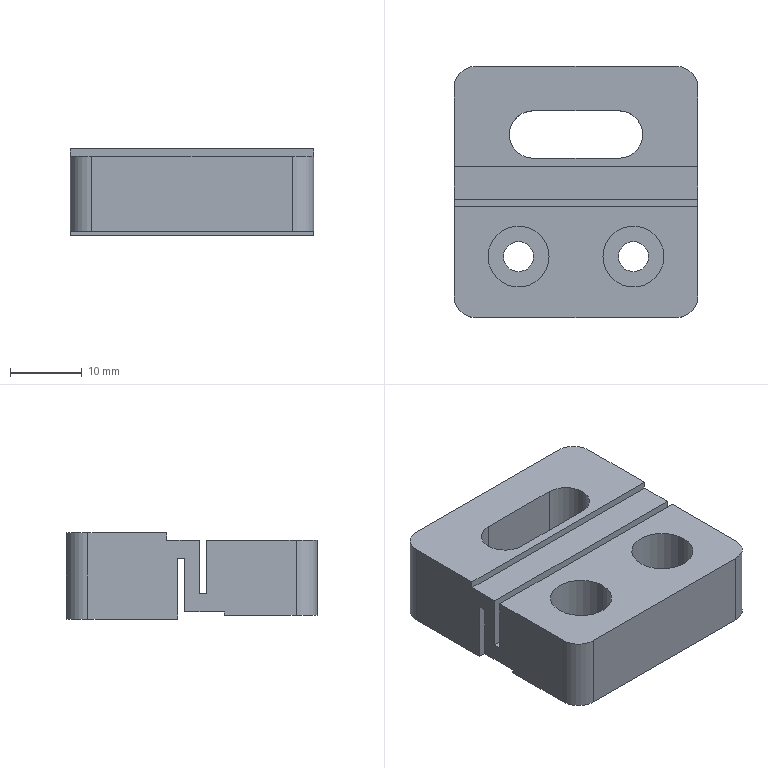Part | SolidWorks | features ICE 7, Extrusion 1, Fillet 1 | 1 solid | 37 faces | box 34 x 35 x 12 mm | volume 10318 mm3 | plane 22 | cylinder 15 | commonest cylinder face diameters 4.2 x4 6 x4 8.5 x4 6.6 x3
STEP:
#1=CARTESIAN_POINT('',(3.75,-9.,4.5));
#2=VERTEX_POINT('',#1);
#3=CARTESIAN_POINT('',(12.25,-9.,4.5));
#4=VERTEX_POINT('',#3);
#5=CARTESIAN_POINT('',(8.,-9.,4.5));
#6=DIRECTION('',(0.,0.,1.));
#7=DIRECTION('',(1.,0.,0.));
#8=AXIS2_PLACEMENT_3D('',#5,#6,#7);
#9=CIRCLE('',#8,4.25);
#10=EDGE_CURVE('',#2,#4,#9,.T.);
#11=ORIENTED_EDGE('',*,*,#10,.F.);
#12=CARTESIAN_POINT('',(3.75,-9.,11.));
#13=VERTEX_POINT('',#12);
#14=CARTESIAN_POINT('',(3.75,-9.,4.5));
#15=DIRECTION('',(0.,0.,1.));
#16=VECTOR('',#15,1000.);
#17=LINE('',#14,#16);
#18=EDGE_CURVE('',#2,#13,#17,.T.);
#19=ORIENTED_EDGE('',*,*,#18,.T.);
#20=CARTESIAN_POINT('',(12.25,-9.,11.));
#21=VERTEX_POINT('',#20);
#22=CARTESIAN_POINT('',(8.,-9.,11.));
#23=DIRECTION('',(0.,0.,1.));
#24=DIRECTION('',(1.,0.,0.));
#25=AXIS2_PLACEMENT_3D('',#22,#23,#24);
#26=CIRCLE('',#25,4.25);
#27=EDGE_CURVE('',#13,#21,#26,.T.);
#28=ORIENTED_EDGE('',*,*,#27,.T.);
#29=CARTESIAN_POINT('',(12.25,-9.,4.5));
#30=DIRECTION('',(0.,0.,1.));
#31=VECTOR('',#30,1000.);
#32=LINE('',#29,#31);
#33=EDGE_CURVE('',#4,#21,#32,.T.);
#34=ORIENTED_EDGE('',*,*,#33,.F.);
#35=EDGE_LOOP('',(#11,#19,#28,#34));
#36=FACE_OUTER_BOUND('',#35,.T.);
#37=CARTESIAN_POINT('',(8.,-9.,4.5));
#38=DIRECTION('',(0.,0.,1.));
#39=DIRECTION('',(1.,0.,0.));
#40=AXIS2_PLACEMENT_3D('',#37,#38,#39);
#41=CYLINDRICAL_SURFACE('',#40,4.25);
#42=ADVANCED_FACE('',(#36),#41,.F.);
#43=CARTESIAN_POINT('',(-12.25,-9.,4.5));
#44=VERTEX_POINT('',#43);
#45=CARTESIAN_POINT('',(-3.75,-9.,4.5));
#46=VERTEX_POINT('',#45);
#47=CARTESIAN_POINT('',(-8.,-9.,4.5));
#48=DIRECTION('',(0.,0.,1.));
#49=DIRECTION('',(1.,0.,0.));
#50=AXIS2_PLACEMENT_3D('',#47,#48,#49);
#51=CIRCLE('',#50,4.25);
#52=EDGE_CURVE('',#44,#46,#51,.T.);
#53=ORIENTED_EDGE('',*,*,#52,.F.);
#54=CARTESIAN_POINT('',(-12.25,-9.,11.));
#55=VERTEX_POINT('',#54);
#56=CARTESIAN_POINT('',(-12.25,-9.,4.5));
#57=DIRECTION('',(0.,0.,1.));
#58=VECTOR('',#57,1000.);
#59=LINE('',#56,#58);
#60=EDGE_CURVE('',#44,#55,#59,.T.);
#61=ORIENTED_EDGE('',*,*,#60,.T.);
#62=CARTESIAN_POINT('',(-3.75,-9.,11.));
#63=VERTEX_POINT('',#62);
#64=CARTESIAN_POINT('',(-8.,-9.,11.));
#65=DIRECTION('',(0.,0.,1.));
#66=DIRECTION('',(1.,0.,0.));
#67=AXIS2_PLACEMENT_3D('',#64,#65,#66);
#68=CIRCLE('',#67,4.25);
#69=EDGE_CURVE('',#55,#63,#68,.T.);
#70=ORIENTED_EDGE('',*,*,#69,.T.);
#71=CARTESIAN_POINT('',(-3.75,-9.,4.5));
#72=DIRECTION('',(0.,0.,1.));
#73=VECTOR('',#72,1000.);
#74=LINE('',#71,#73);
#75=EDGE_CURVE('',#46,#63,#74,.T.);
#76=ORIENTED_EDGE('',*,*,#75,.F.);
#77=EDGE_LOOP('',(#53,#61,#70,#76));
#78=FACE_OUTER_BOUND('',#77,.T.);
#79=CARTESIAN_POINT('',(-8.,-9.,4.5));
#80=DIRECTION('',(0.,0.,1.));
#81=DIRECTION('',(1.,0.,0.));
#82=AXIS2_PLACEMENT_3D('',#79,#80,#81);
#83=CYLINDRICAL_SURFACE('',#82,4.25);
#84=ADVANCED_FACE('',(#78),#83,.F.);
#85=CARTESIAN_POINT('',(9.3,8.,0.));
#86=VERTEX_POINT('',#85);
#87=CARTESIAN_POINT('',(6.,11.3,0.));
#88=VERTEX_POINT('',#87);
#89=CARTESIAN_POINT('',(6.,8.,0.));
#90=DIRECTION('',(0.,0.,1.));
#91=DIRECTION('',(1.,0.,0.));
#92=AXIS2_PLACEMENT_3D('',#89,#90,#91);
#93=CIRCLE('',#92,3.3);
#94=EDGE_CURVE('',#86,#88,#93,.T.);
#95=ORIENTED_EDGE('',*,*,#94,.F.);
#96=CARTESIAN_POINT('',(9.3,8.,12.));
#97=VERTEX_POINT('',#96);
#98=CARTESIAN_POINT('',(9.3,8.,0.));
#99=DIRECTION('',(0.,0.,1.));
#100=VECTOR('',#99,1000.);
#101=LINE('',#98,#100);
#102=EDGE_CURVE('',#86,#97,#101,.T.);
#103=ORIENTED_EDGE('',*,*,#102,.T.);
#104=CARTESIAN_POINT('',(6.,11.3,12.));
#105=VERTEX_POINT('',#104);
#106=CARTESIAN_POINT('',(6.,8.,12.));
#107=DIRECTION('',(0.,0.,1.));
#108=DIRECTION('',(1.,0.,0.));
#109=AXIS2_PLACEMENT_3D('',#106,#107,#108);
#110=CIRCLE('',#109,3.3);
#111=EDGE_CURVE('',#97,#105,#110,.T.);
#112=ORIENTED_EDGE('',*,*,#111,.T.);
#113=CARTESIAN_POINT('',(6.,11.3,0.));
#114=DIRECTION('',(0.,0.,1.));
#115=VECTOR('',#114,1000.);
#116=LINE('',#113,#115);
#117=EDGE_CURVE('',#88,#105,#116,.T.);
#118=ORIENTED_EDGE('',*,*,#117,.F.);
#119=EDGE_LOOP('',(#95,#103,#112,#118));
#120=FACE_OUTER_BOUND('',#119,.T.);
#121=CARTESIAN_POINT('',(6.,8.,0.));
#122=DIRECTION('',(0.,0.,1.));
#123=DIRECTION('',(1.,0.,0.));
#124=AXIS2_PLACEMENT_3D('',#121,#122,#123);
#125=CYLINDRICAL_SURFACE('',#124,3.3);
#126=ADVANCED_FACE('',(#120),#125,.F.);
#127=CARTESIAN_POINT('',(-5.9,-9.,0.5));
#128=VERTEX_POINT('',#127);
#129=CARTESIAN_POINT('',(-10.1,-9.,0.5));
#130=VERTEX_POINT('',#129);
#131=CARTESIAN_POINT('',(-8.,-9.,0.5));
#132=DIRECTION('',(0.,0.,-1.));
#133=DIRECTION('',(1.,0.,0.));
#134=AXIS2_PLACEMENT_3D('',#131,#132,#133);
#135=CIRCLE('',#134,2.1);
#136=EDGE_CURVE('',#128,#130,#135,.T.);
#137=ORIENTED_EDGE('',*,*,#136,.T.);
#138=CARTESIAN_POINT('',(-10.1,-9.,4.5));
#139=VERTEX_POINT('',#138);
#140=CARTESIAN_POINT('',(-10.1,-9.,0.));
#141=DIRECTION('',(0.,0.,1.));
#142=VECTOR('',#141,1000.);
#143=LINE('',#140,#142);
#144=EDGE_CURVE('',#130,#139,#143,.T.);
#145=ORIENTED_EDGE('',*,*,#144,.T.);
#146=CARTESIAN_POINT('',(-5.9,-9.,4.5));
#147=VERTEX_POINT('',#146);
#148=CARTESIAN_POINT('',(-8.,-9.,4.5));
#149=DIRECTION('',(0.,0.,-1.));
#150=DIRECTION('',(1.,0.,0.));
#151=AXIS2_PLACEMENT_3D('',#148,#149,#150);
#152=CIRCLE('',#151,2.1);
#153=EDGE_CURVE('',#147,#139,#152,.T.);
#154=ORIENTED_EDGE('',*,*,#153,.F.);
#155=CARTESIAN_POINT('',(-5.9,-9.,0.));
#156=DIRECTION('',(0.,0.,1.));
#157=VECTOR('',#156,1000.);
#158=LINE('',#155,#157);
#159=EDGE_CURVE('',#128,#147,#158,.T.);
#160=ORIENTED_EDGE('',*,*,#159,.F.);
#161=EDGE_LOOP('',(#137,#145,#154,#160));
#162=FACE_OUTER_BOUND('',#161,.T.);
#163=CARTESIAN_POINT('',(-8.,-9.,0.));
#164=DIRECTION('',(0.,0.,1.));
#165=DIRECTION('',(1.,0.,0.));
#166=AXIS2_PLACEMENT_3D('',#163,#164,#165);
#167=CYLINDRICAL_SURFACE('',#166,2.1);
#168=ADVANCED_FACE('',(#162),#167,.F.);
#169=CARTESIAN_POINT('',(10.1,-9.,0.5));
#170=VERTEX_POINT('',#169);
#171=CARTESIAN_POINT('',(5.9,-9.,0.5));
#172=VERTEX_POINT('',#171);
#173=CARTESIAN_POINT('',(8.,-9.,0.5));
#174=DIRECTION('',(0.,0.,-1.));
#175=DIRECTION('',(1.,0.,0.));
#176=AXIS2_PLACEMENT_3D('',#173,#174,#175);
#177=CIRCLE('',#176,2.1);
#178=EDGE_CURVE('',#170,#172,#177,.T.);
#179=ORIENTED_EDGE('',*,*,#178,.T.);
#180=CARTESIAN_POINT('',(5.9,-9.,4.5));
#181=VERTEX_POINT('',#180);
#182=CARTESIAN_POINT('',(5.9,-9.,0.));
#183=DIRECTION('',(0.,0.,1.));
#184=VECTOR('',#183,1000.);
#185=LINE('',#182,#184);
#186=EDGE_CURVE('',#172,#181,#185,.T.);
#187=ORIENTED_EDGE('',*,*,#186,.T.);
#188=CARTESIAN_POINT('',(10.1,-9.,4.5));
#189=VERTEX_POINT('',#188);
#190=CARTESIAN_POINT('',(8.,-9.,4.5));
#191=DIRECTION('',(0.,0.,-1.));
#192=DIRECTION('',(1.,0.,0.));
#193=AXIS2_PLACEMENT_3D('',#190,#191,#192);
#194=CIRCLE('',#193,2.1);
#195=EDGE_CURVE('',#189,#181,#194,.T.);
#196=ORIENTED_EDGE('',*,*,#195,.F.);
#197=CARTESIAN_POINT('',(10.1,-9.,0.));
#198=DIRECTION('',(0.,0.,1.));
#199=VECTOR('',#198,1000.);
#200=LINE('',#197,#199);
#201=EDGE_CURVE('',#170,#189,#200,.T.);
#202=ORIENTED_EDGE('',*,*,#201,.F.);
#203=EDGE_LOOP('',(#179,#187,#196,#202));
#204=FACE_OUTER_BOUND('',#203,.T.);
#205=CARTESIAN_POINT('',(8.,-9.,0.));
#206=DIRECTION('',(0.,0.,1.));
#207=DIRECTION('',(1.,0.,0.));
#208=AXIS2_PLACEMENT_3D('',#205,#206,#207);
#209=CYLINDRICAL_SURFACE('',#208,2.1);
#210=ADVANCED_FACE('',(#204),#209,.F.);
#211=CARTESIAN_POINT('',(-8.,-9.,11.));
#212=DIRECTION('',(0.,0.,1.));
#213=DIRECTION('',(1.,0.,0.));
#214=AXIS2_PLACEMENT_3D('',#211,#212,#213);
#215=CIRCLE('',#214,4.25);
#216=EDGE_CURVE('',#63,#55,#215,.T.);
#217=ORIENTED_EDGE('',*,*,#216,.F.);
#218=ORIENTED_EDGE('',*,*,#69,.F.);
#219=EDGE_LOOP('',(#217,#218));
#220=FACE_BOUND('',#219,.T.);
#221=CARTESIAN_POINT('',(8.,-9.,11.));
#222=DIRECTION('',(0.,0.,1.));
#223=DIRECTION('',(1.,0.,0.));
#224=AXIS2_PLACEMENT_3D('',#221,#222,#223);
#225=CIRCLE('',#224,4.25);
#226=EDGE_CURVE('',#21,#13,#225,.T.);
#227=ORIENTED_EDGE('',*,*,#226,.F.);
#228=ORIENTED_EDGE('',*,*,#27,.F.);
#229=EDGE_LOOP('',(#227,#228));
#230=FACE_BOUND('',#229,.T.);
#231=CARTESIAN_POINT('',(-17.,-14.5,11.));
#232=VERTEX_POINT('',#231);
#233=CARTESIAN_POINT('',(-17.,-2.,11.));
#234=VERTEX_POINT('',#233);
#235=CARTESIAN_POINT('',(-17.,-17.5,11.));
#236=DIRECTION('',(0.,1.,0.));
#237=VECTOR('',#236,1000.);
#238=LINE('',#235,#237);
#239=EDGE_CURVE('',#232,#234,#238,.T.);
#240=ORIENTED_EDGE('',*,*,#239,.F.);
#241=CARTESIAN_POINT('',(-14.,-17.5,11.));
#242=VERTEX_POINT('',#241);
#243=CARTESIAN_POINT('',(-14.,-14.5,11.));
#244=DIRECTION('',(0.,0.,1.));
#245=DIRECTION('',(-1.,0.,0.));
#246=AXIS2_PLACEMENT_3D('',#243,#244,#245);
#247=CIRCLE('',#246,3.);
#248=EDGE_CURVE('',#232,#242,#247,.T.);
#249=ORIENTED_EDGE('',*,*,#248,.T.);
#250=CARTESIAN_POINT('',(14.,-17.5,11.));
#251=VERTEX_POINT('',#250);
#252=CARTESIAN_POINT('',(17.,-17.5,11.));
#253=DIRECTION('',(-1.,0.,0.));
#254=VECTOR('',#253,1000.);
#255=LINE('',#252,#254);
#256=EDGE_CURVE('',#251,#242,#255,.T.);
#257=ORIENTED_EDGE('',*,*,#256,.F.);
#258=CARTESIAN_POINT('',(17.,-14.5,11.));
#259=VERTEX_POINT('',#258);
#260=CARTESIAN_POINT('',(14.,-14.5,11.));
#261=DIRECTION('',(0.,0.,1.));
#262=DIRECTION('',(-1.,0.,0.));
#263=AXIS2_PLACEMENT_3D('',#260,#261,#262);
#264=CIRCLE('',#263,3.);
#265=EDGE_CURVE('',#251,#259,#264,.T.);
#266=ORIENTED_EDGE('',*,*,#265,.T.);
#267=CARTESIAN_POINT('',(17.,-2.,11.));
#268=VERTEX_POINT('',#267);
#269=CARTESIAN_POINT('',(17.,-17.5,11.));
#270=DIRECTION('',(0.,-1.,0.));
#271=VECTOR('',#270,1000.);
#272=LINE('',#269,#271);
#273=EDGE_CURVE('',#268,#259,#272,.T.);
#274=ORIENTED_EDGE('',*,*,#273,.F.);
#275=CARTESIAN_POINT('',(17.,-2.,11.));
#276=DIRECTION('',(1.,0.,0.));
#277=VECTOR('',#276,1000.);
#278=LINE('',#275,#277);
#279=EDGE_CURVE('',#234,#268,#278,.T.);
#280=ORIENTED_EDGE('',*,*,#279,.F.);
#281=EDGE_LOOP('',(#240,#249,#257,#266,#274,#280));
#282=FACE_OUTER_BOUND('',#281,.T.);
#283=CARTESIAN_POINT('',(0.,0.,11.));
#284=DIRECTION('',(0.,0.,-1.));
#285=DIRECTION('',(-1.,0.,0.));
#286=AXIS2_PLACEMENT_3D('',#283,#284,#285);
#287=PLANE('',#286);
#288=ADVANCED_FACE('',(#220,#230,#282),#287,.F.);
#289=ORIENTED_EDGE('',*,*,#186,.F.);
#290=CARTESIAN_POINT('',(8.,-9.,0.5));
#291=DIRECTION('',(0.,0.,-1.));
#292=DIRECTION('',(1.,0.,0.));
#293=AXIS2_PLACEMENT_3D('',#290,#291,#292);
#294=CIRCLE('',#293,2.1);
#295=EDGE_CURVE('',#172,#170,#294,.T.);
#296=ORIENTED_EDGE('',*,*,#295,.T.);
#297=ORIENTED_EDGE('',*,*,#201,.T.);
#298=CARTESIAN_POINT('',(8.,-9.,4.5));
#299=DIRECTION('',(0.,0.,-1.));
#300=DIRECTION('',(1.,0.,0.));
#301=AXIS2_PLACEMENT_3D('',#298,#299,#300);
#302=CIRCLE('',#301,2.1);
#303=EDGE_CURVE('',#181,#189,#302,.T.);
#304=ORIENTED_EDGE('',*,*,#303,.F.);
#305=EDGE_LOOP('',(#289,#296,#297,#304));
#306=FACE_OUTER_BOUND('',#305,.T.);
#307=CARTESIAN_POINT('',(8.,-9.,0.));
#308=DIRECTION('',(0.,0.,1.));
#309=DIRECTION('',(1.,0.,0.));
#310=AXIS2_PLACEMENT_3D('',#307,#308,#309);
#311=CYLINDRICAL_SURFACE('',#310,2.1);
#312=ADVANCED_FACE('',(#306),#311,.F.);
#313=ORIENTED_EDGE('',*,*,#144,.F.);
#314=CARTESIAN_POINT('',(-8.,-9.,0.5));
#315=DIRECTION('',(0.,0.,-1.));
#316=DIRECTION('',(1.,0.,0.));
#317=AXIS2_PLACEMENT_3D('',#314,#315,#316);
#318=CIRCLE('',#317,2.1);
#319=EDGE_CURVE('',#130,#128,#318,.T.);
#320=ORIENTED_EDGE('',*,*,#319,.T.);
#321=ORIENTED_EDGE('',*,*,#159,.T.);
#322=CARTESIAN_POINT('',(-8.,-9.,4.5));
#323=DIRECTION('',(0.,0.,-1.));
#324=DIRECTION('',(1.,0.,0.));
#325=AXIS2_PLACEMENT_3D('',#322,#323,#324);
#326=CIRCLE('',#325,2.1);
#327=EDGE_CURVE('',#139,#147,#326,.T.);
#328=ORIENTED_EDGE('',*,*,#327,.F.);
#329=EDGE_LOOP('',(#313,#320,#321,#328));
#330=FACE_OUTER_BOUND('',#329,.T.);
#331=CARTESIAN_POINT('',(-8.,-9.,0.));
#332=DIRECTION('',(0.,0.,1.));
#333=DIRECTION('',(1.,0.,0.));
#334=AXIS2_PLACEMENT_3D('',#331,#332,#333);
#335=CYLINDRICAL_SURFACE('',#334,2.1);
#336=ADVANCED_FACE('',(#330),#335,.F.);
#337=CARTESIAN_POINT('',(-17.,-4.5,0.5));
#338=VERTEX_POINT('',#337);
#339=CARTESIAN_POINT('',(-17.,-14.5,0.5));
#340=VERTEX_POINT('',#339);
#341=CARTESIAN_POINT('',(-17.,-17.5,0.5));
#342=DIRECTION('',(0.,-1.,0.));
#343=VECTOR('',#342,1000.);
#344=LINE('',#341,#343);
#345=EDGE_CURVE('',#338,#340,#344,.T.);
#346=ORIENTED_EDGE('',*,*,#345,.T.);
#347=CARTESIAN_POINT('',(-17.,-14.5,12.));
#348=DIRECTION('',(0.,0.,1.));
#349=VECTOR('',#348,1000.);
#350=LINE('',#347,#349);
#351=EDGE_CURVE('',#340,#232,#350,.T.);
#352=ORIENTED_EDGE('',*,*,#351,.T.);
#353=ORIENTED_EDGE('',*,*,#239,.T.);
#354=CARTESIAN_POINT('',(-17.,-2.,3.5));
#355=VERTEX_POINT('',#354);
#356=CARTESIAN_POINT('',(-17.,-2.,-33.015));
#357=DIRECTION('',(0.,0.,1.));
#358=VECTOR('',#357,1000.);
#359=LINE('',#356,#358);
#360=EDGE_CURVE('',#355,#234,#359,.T.);
#361=ORIENTED_EDGE('',*,*,#360,.F.);
#362=CARTESIAN_POINT('',(-17.,-1.,3.5));
#363=VERTEX_POINT('',#362);
#364=CARTESIAN_POINT('',(-17.,-2.,3.5));
#365=DIRECTION('',(0.,1.,0.));
#366=VECTOR('',#365,1000.);
#367=LINE('',#364,#366);
#368=EDGE_CURVE('',#355,#363,#367,.T.);
#369=ORIENTED_EDGE('',*,*,#368,.T.);
#370=CARTESIAN_POINT('',(-17.,-1.,11.));
#371=VERTEX_POINT('',#370);
#372=CARTESIAN_POINT('',(-17.,-1.,-33.015));
#373=DIRECTION('',(0.,0.,1.));
#374=VECTOR('',#373,1000.);
#375=LINE('',#372,#374);
#376=EDGE_CURVE('',#363,#371,#375,.T.);
#377=ORIENTED_EDGE('',*,*,#376,.T.);
#378=CARTESIAN_POINT('',(-17.,3.5,11.));
#379=VERTEX_POINT('',#378);
#380=CARTESIAN_POINT('',(-17.,-17.5,11.));
#381=DIRECTION('',(0.,1.,0.));
#382=VECTOR('',#381,1000.);
#383=LINE('',#380,#382);
#384=EDGE_CURVE('',#371,#379,#383,.T.);
#385=ORIENTED_EDGE('',*,*,#384,.T.);
#386=CARTESIAN_POINT('',(-17.,3.5,12.));
#387=VERTEX_POINT('',#386);
#388=CARTESIAN_POINT('',(-17.,3.5,12.));
#389=DIRECTION('',(0.,0.,1.));
#390=VECTOR('',#389,1000.);
#391=LINE('',#388,#390);
#392=EDGE_CURVE('',#379,#387,#391,.T.);
#393=ORIENTED_EDGE('',*,*,#392,.T.);
#394=CARTESIAN_POINT('',(-17.,14.5,12.));
#395=VERTEX_POINT('',#394);
#396=CARTESIAN_POINT('',(-17.,-17.5,12.));
#397=DIRECTION('',(0.,-1.,0.));
#398=VECTOR('',#397,1000.);
#399=LINE('',#396,#398);
#400=EDGE_CURVE('',#395,#387,#399,.T.);
#401=ORIENTED_EDGE('',*,*,#400,.F.);
#402=CARTESIAN_POINT('',(-17.,14.5,0.));
#403=VERTEX_POINT('',#402);
#404=CARTESIAN_POINT('',(-17.,14.5,12.));
#405=DIRECTION('',(0.,0.,-1.));
#406=VECTOR('',#405,1000.);
#407=LINE('',#404,#406);
#408=EDGE_CURVE('',#395,#403,#407,.T.);
#409=ORIENTED_EDGE('',*,*,#408,.T.);
#410=CARTESIAN_POINT('',(-17.,2.,0.));
#411=VERTEX_POINT('',#410);
#412=CARTESIAN_POINT('',(-17.,-17.5,0.));
#413=DIRECTION('',(0.,-1.,0.));
#414=VECTOR('',#413,1000.);
#415=LINE('',#412,#414);
#416=EDGE_CURVE('',#403,#411,#415,.T.);
#417=ORIENTED_EDGE('',*,*,#416,.T.);
#418=CARTESIAN_POINT('',(-17.,2.,8.5));
#419=VERTEX_POINT('',#418);
#420=CARTESIAN_POINT('',(-17.,2.,12.));
#421=DIRECTION('',(0.,0.,1.));
#422=VECTOR('',#421,1000.);
#423=LINE('',#420,#422);
#424=EDGE_CURVE('',#411,#419,#423,.T.);
#425=ORIENTED_EDGE('',*,*,#424,.T.);
#426=CARTESIAN_POINT('',(-17.,1.,8.5));
#427=VERTEX_POINT('',#426);
#428=CARTESIAN_POINT('',(-17.,2.,8.5));
#429=DIRECTION('',(0.,-1.,0.));
#430=VECTOR('',#429,1000.);
#431=LINE('',#428,#430);
#432=EDGE_CURVE('',#419,#427,#431,.T.);
#433=ORIENTED_EDGE('',*,*,#432,.T.);
#434=CARTESIAN_POINT('',(-17.,1.,1.));
#435=VERTEX_POINT('',#434);
#436=CARTESIAN_POINT('',(-17.,1.,46.635));
#437=DIRECTION('',(0.,0.,-1.));
#438=VECTOR('',#437,1000.);
#439=LINE('',#436,#438);
#440=EDGE_CURVE('',#427,#435,#439,.T.);
#441=ORIENTED_EDGE('',*,*,#440,.T.);
#442=CARTESIAN_POINT('',(-17.,-4.5,1.));
#443=VERTEX_POINT('',#442);
#444=CARTESIAN_POINT('',(-17.,-17.5,1.));
#445=DIRECTION('',(0.,-1.,0.));
#446=VECTOR('',#445,1000.);
#447=LINE('',#444,#446);
#448=EDGE_CURVE('',#435,#443,#447,.T.);
#449=ORIENTED_EDGE('',*,*,#448,.T.);
#450=CARTESIAN_POINT('',(-17.,-4.5,1.));
#451=DIRECTION('',(0.,0.,-1.));
#452=VECTOR('',#451,1000.);
#453=LINE('',#450,#452);
#454=EDGE_CURVE('',#443,#338,#453,.T.);
#455=ORIENTED_EDGE('',*,*,#454,.T.);
#456=EDGE_LOOP('',(#346,#352,#353,#361,#369,#377,#385,#393,#401,#409,#417,#425,#433,#441,#449,#455));
#457=FACE_OUTER_BOUND('',#456,.T.);
#458=CARTESIAN_POINT('',(-17.,-17.5,12.));
#459=DIRECTION('',(1.,0.,0.));
#460=DIRECTION('',(0.,0.,-1.));
#461=AXIS2_PLACEMENT_3D('',#458,#459,#460);
#462=PLANE('',#461);
#463=ADVANCED_FACE('',(#457),#462,.F.);
#464=ORIENTED_EDGE('',*,*,#256,.T.);
#465=CARTESIAN_POINT('',(-14.,-17.5,0.5));
#466=VERTEX_POINT('',#465);
#467=CARTESIAN_POINT('',(-14.,-17.5,12.));
#468=DIRECTION('',(0.,0.,-1.));
#469=VECTOR('',#468,1000.);
#470=LINE('',#467,#469);
#471=EDGE_CURVE('',#242,#466,#470,.T.);
#472=ORIENTED_EDGE('',*,*,#471,.T.);
#473=CARTESIAN_POINT('',(14.,-17.5,0.5));
#474=VERTEX_POINT('',#473);
#475=CARTESIAN_POINT('',(17.,-17.5,0.5));
#476=DIRECTION('',(1.,0.,0.));
#477=VECTOR('',#476,1000.);
#478=LINE('',#475,#477);
#479=EDGE_CURVE('',#466,#474,#478,.T.);
#480=ORIENTED_EDGE('',*,*,#479,.T.);
#481=CARTESIAN_POINT('',(14.,-17.5,12.));
#482=DIRECTION('',(0.,0.,1.));
#483=VECTOR('',#482,1000.);
#484=LINE('',#481,#483);
#485=EDGE_CURVE('',#474,#251,#484,.T.);
#486=ORIENTED_EDGE('',*,*,#485,.T.);
#487=EDGE_LOOP('',(#464,#472,#480,#486));
#488=FACE_OUTER_BOUND('',#487,.T.);
#489=CARTESIAN_POINT('',(17.,-17.5,12.));
#490=DIRECTION('',(0.,1.,0.));
#491=DIRECTION('',(-1.,0.,0.));
#492=AXIS2_PLACEMENT_3D('',#489,#490,#491);
#493=PLANE('',#492);
#494=ADVANCED_FACE('',(#488),#493,.F.);
#495=ORIENTED_EDGE('',*,*,#273,.T.);
#496=CARTESIAN_POINT('',(17.,-14.5,0.5));
#497=VERTEX_POINT('',#496);
#498=CARTESIAN_POINT('',(17.,-14.5,12.));
#499=DIRECTION('',(0.,0.,-1.));
#500=VECTOR('',#499,1000.);
#501=LINE('',#498,#500);
#502=EDGE_CURVE('',#259,#497,#501,.T.);
#503=ORIENTED_EDGE('',*,*,#502,.T.);
#504=CARTESIAN_POINT('',(17.,-4.5,0.5));
#505=VERTEX_POINT('',#504);
#506=CARTESIAN_POINT('',(17.,-17.5,0.5));
#507=DIRECTION('',(0.,1.,0.));
#508=VECTOR('',#507,1000.);
#509=LINE('',#506,#508);
#510=EDGE_CURVE('',#497,#505,#509,.T.);
#511=ORIENTED_EDGE('',*,*,#510,.T.);
#512=CARTESIAN_POINT('',(17.,-4.5,1.));
#513=VERTEX_POINT('',#512);
#514=CARTESIAN_POINT('',(17.,-4.5,1.));
#515=DIRECTION('',(0.,0.,-1.));
#516=VECTOR('',#515,1000.);
#517=LINE('',#514,#516);
#518=EDGE_CURVE('',#513,#505,#517,.T.);
#519=ORIENTED_EDGE('',*,*,#518,.F.);
#520=CARTESIAN_POINT('',(17.,1.,1.));
#521=VERTEX_POINT('',#520);
#522=CARTESIAN_POINT('',(17.,-17.5,1.));
#523=DIRECTION('',(0.,1.,0.));
#524=VECTOR('',#523,1000.);
#525=LINE('',#522,#524);
#526=EDGE_CURVE('',#513,#521,#525,.T.);
#527=ORIENTED_EDGE('',*,*,#526,.T.);
#528=CARTESIAN_POINT('',(17.,1.,8.5));
#529=VERTEX_POINT('',#528);
#530=CARTESIAN_POINT('',(17.,1.,12.));
#531=DIRECTION('',(0.,0.,1.));
#532=VECTOR('',#531,1000.);
#533=LINE('',#530,#532);
#534=EDGE_CURVE('',#521,#529,#533,.T.);
#535=ORIENTED_EDGE('',*,*,#534,.T.);
#536=CARTESIAN_POINT('',(17.,2.,8.5));
#537=VERTEX_POINT('',#536);
#538=CARTESIAN_POINT('',(17.,-17.5,8.5));
#539=DIRECTION('',(0.,-1.,0.));
#540=VECTOR('',#539,1000.);
#541=LINE('',#538,#540);
#542=EDGE_CURVE('',#537,#529,#541,.T.);
#543=ORIENTED_EDGE('',*,*,#542,.F.);
#544=CARTESIAN_POINT('',(17.,2.,0.));
#545=VERTEX_POINT('',#544);
#546=CARTESIAN_POINT('',(17.,2.,12.));
#547=DIRECTION('',(0.,0.,-1.));
#548=VECTOR('',#547,1000.);
#549=LINE('',#546,#548);
#550=EDGE_CURVE('',#537,#545,#549,.T.);
#551=ORIENTED_EDGE('',*,*,#550,.T.);
#552=CARTESIAN_POINT('',(17.,14.5,0.));
#553=VERTEX_POINT('',#552);
#554=CARTESIAN_POINT('',(17.,-17.5,0.));
#555=DIRECTION('',(0.,1.,0.));
#556=VECTOR('',#555,1000.);
#557=LINE('',#554,#556);
#558=EDGE_CURVE('',#545,#553,#557,.T.);
#559=ORIENTED_EDGE('',*,*,#558,.T.);
#560=CARTESIAN_POINT('',(17.,14.5,12.));
#561=VERTEX_POINT('',#560);
#562=CARTESIAN_POINT('',(17.,14.5,12.));
#563=DIRECTION('',(0.,0.,1.));
#564=VECTOR('',#563,1000.);
#565=LINE('',#562,#564);
#566=EDGE_CURVE('',#553,#561,#565,.T.);
#567=ORIENTED_EDGE('',*,*,#566,.T.);
#568=CARTESIAN_POINT('',(17.,3.5,12.));
#569=VERTEX_POINT('',#568);
#570=CARTESIAN_POINT('',(17.,-17.5,12.));
#571=DIRECTION('',(0.,1.,0.));
#572=VECTOR('',#571,1000.);
#573=LINE('',#570,#572);
#574=EDGE_CURVE('',#569,#561,#573,.T.);
#575=ORIENTED_EDGE('',*,*,#574,.F.);
#576=CARTESIAN_POINT('',(17.,3.5,11.));
#577=VERTEX_POINT('',#576);
#578=CARTESIAN_POINT('',(17.,3.5,12.));
#579=DIRECTION('',(0.,0.,-1.));
#580=VECTOR('',#579,1000.);
#581=LINE('',#578,#580);
#582=EDGE_CURVE('',#569,#577,#581,.T.);
#583=ORIENTED_EDGE('',*,*,#582,.T.);
#584=CARTESIAN_POINT('',(17.,-1.,11.));
#585=VERTEX_POINT('',#584);
#586=CARTESIAN_POINT('',(17.,-17.5,11.));
#587=DIRECTION('',(0.,-1.,0.));
#588=VECTOR('',#587,1000.);
#589=LINE('',#586,#588);
#590=EDGE_CURVE('',#577,#585,#589,.T.);
#591=ORIENTED_EDGE('',*,*,#590,.T.);
#592=CARTESIAN_POINT('',(17.,-1.,3.5));
#593=VERTEX_POINT('',#592);
#594=CARTESIAN_POINT('',(17.,-1.,-33.015));
#595=DIRECTION('',(0.,0.,1.));
#596=VECTOR('',#595,1000.);
#597=LINE('',#594,#596);
#598=EDGE_CURVE('',#593,#585,#597,.T.);
#599=ORIENTED_EDGE('',*,*,#598,.F.);
#600=CARTESIAN_POINT('',(17.,-2.,3.5));
#601=VERTEX_POINT('',#600);
#602=CARTESIAN_POINT('',(17.,-1.,3.5));
#603=DIRECTION('',(0.,-1.,0.));
#604=VECTOR('',#603,1000.);
#605=LINE('',#602,#604);
#606=EDGE_CURVE('',#593,#601,#605,.T.);
#607=ORIENTED_EDGE('',*,*,#606,.T.);
#608=CARTESIAN_POINT('',(17.,-2.,-33.015));
#609=DIRECTION('',(0.,0.,1.));
#610=VECTOR('',#609,1000.);
#611=LINE('',#608,#610);
#612=EDGE_CURVE('',#601,#268,#611,.T.);
#613=ORIENTED_EDGE('',*,*,#612,.T.);
#614=EDGE_LOOP('',(#495,#503,#511,#519,#527,#535,#543,#551,#559,#567,#575,#583,#591,#599,#607,#613));
#615=FACE_OUTER_BOUND('',#614,.T.);
#616=CARTESIAN_POINT('',(17.,-17.5,12.));
#617=DIRECTION('',(-1.,0.,0.));
#618=DIRECTION('',(0.,0.,1.));
#619=AXIS2_PLACEMENT_3D('',#616,#617,#618);
#620=PLANE('',#619);
#621=ADVANCED_FACE('',(#615),#620,.F.);
#622=CARTESIAN_POINT('',(14.,17.5,12.));
#623=VERTEX_POINT('',#622);
#624=CARTESIAN_POINT('',(-14.,17.5,12.));
#625=VERTEX_POINT('',#624);
#626=CARTESIAN_POINT('',(17.,17.5,12.));
#627=DIRECTION('',(-1.,0.,0.));
#628=VECTOR('',#627,1000.);
#629=LINE('',#626,#628);
#630=EDGE_CURVE('',#623,#625,#629,.T.);
#631=ORIENTED_EDGE('',*,*,#630,.F.);
#632=CARTESIAN_POINT('',(14.,17.5,0.));
#633=VERTEX_POINT('',#632);
#634=CARTESIAN_POINT('',(14.,17.5,12.));
#635=DIRECTION('',(0.,0.,-1.));
#636=VECTOR('',#635,1000.);
#637=LINE('',#634,#636);
#638=EDGE_CURVE('',#623,#633,#637,.T.);
#639=ORIENTED_EDGE('',*,*,#638,.T.);
#640=CARTESIAN_POINT('',(-14.,17.5,0.));
#641=VERTEX_POINT('',#640);
#642=CARTESIAN_POINT('',(17.,17.5,0.));
#643=DIRECTION('',(-1.,0.,0.));
#644=VECTOR('',#643,1000.);
#645=LINE('',#642,#644);
#646=EDGE_CURVE('',#633,#641,#645,.T.);
#647=ORIENTED_EDGE('',*,*,#646,.T.);
#648=CARTESIAN_POINT('',(-14.,17.5,12.));
#649=DIRECTION('',(0.,0.,1.));
#650=VECTOR('',#649,1000.);
#651=LINE('',#648,#650);
#652=EDGE_CURVE('',#641,#625,#651,.T.);
#653=ORIENTED_EDGE('',*,*,#652,.T.);
#654=EDGE_LOOP('',(#631,#639,#647,#653));
#655=FACE_OUTER_BOUND('',#654,.T.);
#656=CARTESIAN_POINT('',(17.,17.5,12.));
#657=DIRECTION('',(0.,-1.,0.));
#658=DIRECTION('',(0.,0.,-1.));
#659=AXIS2_PLACEMENT_3D('',#656,#657,#658);
#660=PLANE('',#659);
#661=ADVANCED_FACE('',(#655),#660,.F.);
#662=ORIENTED_EDGE('',*,*,#574,.T.);
#663=CARTESIAN_POINT('',(14.,14.5,12.));
#664=DIRECTION('',(0.,0.,1.));
#665=DIRECTION('',(1.,0.,0.));
#666=AXIS2_PLACEMENT_3D('',#663,#664,#665);
#667=CIRCLE('',#666,3.);
#668=EDGE_CURVE('',#561,#623,#667,.T.);
#669=ORIENTED_EDGE('',*,*,#668,.T.);
#670=ORIENTED_EDGE('',*,*,#630,.T.);
#671=CARTESIAN_POINT('',(-14.,14.5,12.));
#672=DIRECTION('',(0.,0.,1.));
#673=DIRECTION('',(1.,0.,0.));
#674=AXIS2_PLACEMENT_3D('',#671,#672,#673);
#675=CIRCLE('',#674,3.);
#676=EDGE_CURVE('',#625,#395,#675,.T.);
#677=ORIENTED_EDGE('',*,*,#676,.T.);
#678=ORIENTED_EDGE('',*,*,#400,.T.);
#679=CARTESIAN_POINT('',(-20.364,3.5,12.));
#680=DIRECTION('',(-1.,0.,0.));
#681=VECTOR('',#680,1000.);
#682=LINE('',#679,#681);
#683=EDGE_CURVE('',#569,#387,#682,.T.);
#684=ORIENTED_EDGE('',*,*,#683,.F.);
#685=EDGE_LOOP('',(#662,#669,#670,#677,#678,#684));
#686=FACE_OUTER_BOUND('',#685,.T.);
#687=CARTESIAN_POINT('',(-6.,11.3,12.));
#688=VERTEX_POINT('',#687);
#689=CARTESIAN_POINT('',(-6.,4.7,12.));
#690=VERTEX_POINT('',#689);
#691=CARTESIAN_POINT('',(-6.,8.,12.));
#692=DIRECTION('',(0.,0.,1.));
#693=DIRECTION('',(1.,0.,0.));
#694=AXIS2_PLACEMENT_3D('',#691,#692,#693);
#695=CIRCLE('',#694,3.3);
#696=EDGE_CURVE('',#688,#690,#695,.T.);
#697=ORIENTED_EDGE('',*,*,#696,.F.);
#698=CARTESIAN_POINT('',(-6.,11.3,12.));
#699=DIRECTION('',(-1.,0.,0.));
#700=VECTOR('',#699,1000.);
#701=LINE('',#698,#700);
#702=EDGE_CURVE('',#105,#688,#701,.T.);
#703=ORIENTED_EDGE('',*,*,#702,.F.);
#704=ORIENTED_EDGE('',*,*,#111,.F.);
#705=CARTESIAN_POINT('',(6.,4.7,12.));
#706=VERTEX_POINT('',#705);
#707=CARTESIAN_POINT('',(6.,8.,12.));
#708=DIRECTION('',(0.,0.,1.));
#709=DIRECTION('',(1.,0.,0.));
#710=AXIS2_PLACEMENT_3D('',#707,#708,#709);
#711=CIRCLE('',#710,3.3);
#712=EDGE_CURVE('',#706,#97,#711,.T.);
#713=ORIENTED_EDGE('',*,*,#712,.F.);
#714=CARTESIAN_POINT('',(-6.,4.7,12.));
#715=DIRECTION('',(1.,0.,0.));
#716=VECTOR('',#715,1000.);
#717=LINE('',#714,#716);
#718=EDGE_CURVE('',#690,#706,#717,.T.);
#719=ORIENTED_EDGE('',*,*,#718,.F.);
#720=EDGE_LOOP('',(#697,#703,#704,#713,#719));
#721=FACE_BOUND('',#720,.T.);
#722=CARTESIAN_POINT('',(0.,0.,12.));
#723=DIRECTION('',(0.,0.,1.));
#724=DIRECTION('',(1.,0.,0.));
#725=AXIS2_PLACEMENT_3D('',#722,#723,#724);
#726=PLANE('',#725);
#727=ADVANCED_FACE('',(#686,#721),#726,.T.);
#728=CARTESIAN_POINT('',(-6.,11.3,0.));
#729=VERTEX_POINT('',#728);
#730=CARTESIAN_POINT('',(-6.,11.3,0.));
#731=DIRECTION('',(-1.,0.,0.));
#732=VECTOR('',#731,1000.);
#733=LINE('',#730,#732);
#734=EDGE_CURVE('',#88,#729,#733,.T.);
#735=ORIENTED_EDGE('',*,*,#734,.T.);
#736=CARTESIAN_POINT('',(-6.,4.7,0.));
#737=VERTEX_POINT('',#736);
#738=CARTESIAN_POINT('',(-6.,8.,0.));
#739=DIRECTION('',(0.,0.,1.));
#740=DIRECTION('',(1.,0.,0.));
#741=AXIS2_PLACEMENT_3D('',#738,#739,#740);
#742=CIRCLE('',#741,3.3);
#743=EDGE_CURVE('',#729,#737,#742,.T.);
#744=ORIENTED_EDGE('',*,*,#743,.T.);
#745=CARTESIAN_POINT('',(6.,4.7,0.));
#746=VERTEX_POINT('',#745);
#747=CARTESIAN_POINT('',(-6.,4.7,0.));
#748=DIRECTION('',(1.,0.,0.));
#749=VECTOR('',#748,1000.);
#750=LINE('',#747,#749);
#751=EDGE_CURVE('',#737,#746,#750,.T.);
#752=ORIENTED_EDGE('',*,*,#751,.T.);
#753=CARTESIAN_POINT('',(6.,8.,0.));
#754=DIRECTION('',(0.,0.,1.));
#755=DIRECTION('',(1.,0.,0.));
#756=AXIS2_PLACEMENT_3D('',#753,#754,#755);
#757=CIRCLE('',#756,3.3);
#758=EDGE_CURVE('',#746,#86,#757,.T.);
#759=ORIENTED_EDGE('',*,*,#758,.T.);
#760=ORIENTED_EDGE('',*,*,#94,.T.);
#761=EDGE_LOOP('',(#735,#744,#752,#759,#760));
#762=FACE_BOUND('',#761,.T.);
#763=ORIENTED_EDGE('',*,*,#646,.F.);
#764=CARTESIAN_POINT('',(14.,14.5,0.));
#765=DIRECTION('',(0.,0.,-1.));
#766=DIRECTION('',(1.,0.,0.));
#767=AXIS2_PLACEMENT_3D('',#764,#765,#766);
#768=CIRCLE('',#767,3.);
#769=EDGE_CURVE('',#633,#553,#768,.T.);
#770=ORIENTED_EDGE('',*,*,#769,.T.);
#771=ORIENTED_EDGE('',*,*,#558,.F.);
#772=CARTESIAN_POINT('',(23.913,2.,0.));
#773=DIRECTION('',(1.,0.,0.));
#774=VECTOR('',#773,1000.);
#775=LINE('',#772,#774);
#776=EDGE_CURVE('',#411,#545,#775,.T.);
#777=ORIENTED_EDGE('',*,*,#776,.F.);
#778=ORIENTED_EDGE('',*,*,#416,.F.);
#779=CARTESIAN_POINT('',(-14.,14.5,0.));
#780=DIRECTION('',(0.,0.,-1.));
#781=DIRECTION('',(1.,0.,0.));
#782=AXIS2_PLACEMENT_3D('',#779,#780,#781);
#783=CIRCLE('',#782,3.);
#784=EDGE_CURVE('',#403,#641,#783,.T.);
#785=ORIENTED_EDGE('',*,*,#784,.T.);
#786=EDGE_LOOP('',(#763,#770,#771,#777,#778,#785));
#787=FACE_OUTER_BOUND('',#786,.T.);
#788=CARTESIAN_POINT('',(0.,0.,0.));
#789=DIRECTION('',(0.,0.,1.));
#790=DIRECTION('',(1.,0.,0.));
#791=AXIS2_PLACEMENT_3D('',#788,#789,#790);
#792=PLANE('',#791);
#793=ADVANCED_FACE('',(#762,#787),#792,.F.);
#794=ORIENTED_EDGE('',*,*,#696,.T.);
#795=CARTESIAN_POINT('',(-6.,4.7,0.));
#796=DIRECTION('',(0.,0.,1.));
#797=VECTOR('',#796,1000.);
#798=LINE('',#795,#797);
#799=EDGE_CURVE('',#737,#690,#798,.T.);
#800=ORIENTED_EDGE('',*,*,#799,.F.);
#801=ORIENTED_EDGE('',*,*,#743,.F.);
#802=CARTESIAN_POINT('',(-6.,11.3,0.));
#803=DIRECTION('',(0.,0.,1.));
#804=VECTOR('',#803,1000.);
#805=LINE('',#802,#804);
#806=EDGE_CURVE('',#729,#688,#805,.T.);
#807=ORIENTED_EDGE('',*,*,#806,.T.);
#808=EDGE_LOOP('',(#794,#800,#801,#807));
#809=FACE_OUTER_BOUND('',#808,.T.);
#810=CARTESIAN_POINT('',(-6.,8.,0.));
#811=DIRECTION('',(0.,0.,1.));
#812=DIRECTION('',(1.,0.,0.));
#813=AXIS2_PLACEMENT_3D('',#810,#811,#812);
#814=CYLINDRICAL_SURFACE('',#813,3.3);
#815=ADVANCED_FACE('',(#809),#814,.F.);
#816=ORIENTED_EDGE('',*,*,#702,.T.);
#817=ORIENTED_EDGE('',*,*,#806,.F.);
#818=ORIENTED_EDGE('',*,*,#734,.F.);
#819=ORIENTED_EDGE('',*,*,#117,.T.);
#820=EDGE_LOOP('',(#816,#817,#818,#819));
#821=FACE_OUTER_BOUND('',#820,.T.);
#822=CARTESIAN_POINT('',(-6.,11.3,0.));
#823=DIRECTION('',(0.,1.,0.));
#824=DIRECTION('',(0.,0.,1.));
#825=AXIS2_PLACEMENT_3D('',#822,#823,#824);
#826=PLANE('',#825);
#827=ADVANCED_FACE('',(#821),#826,.F.);
#828=ORIENTED_EDGE('',*,*,#102,.F.);
#829=ORIENTED_EDGE('',*,*,#758,.F.);
#830=CARTESIAN_POINT('',(6.,4.7,0.));
#831=DIRECTION('',(0.,0.,1.));
#832=VECTOR('',#831,1000.);
#833=LINE('',#830,#832);
#834=EDGE_CURVE('',#746,#706,#833,.T.);
#835=ORIENTED_EDGE('',*,*,#834,.T.);
#836=ORIENTED_EDGE('',*,*,#712,.T.);
#837=EDGE_LOOP('',(#828,#829,#835,#836));
#838=FACE_OUTER_BOUND('',#837,.T.);
#839=CARTESIAN_POINT('',(6.,8.,0.));
#840=DIRECTION('',(0.,0.,1.));
#841=DIRECTION('',(1.,0.,0.));
#842=AXIS2_PLACEMENT_3D('',#839,#840,#841);
#843=CYLINDRICAL_SURFACE('',#842,3.3);
#844=ADVANCED_FACE('',(#838),#843,.F.);
#845=ORIENTED_EDGE('',*,*,#718,.T.);
#846=ORIENTED_EDGE('',*,*,#834,.F.);
#847=ORIENTED_EDGE('',*,*,#751,.F.);
#848=ORIENTED_EDGE('',*,*,#799,.T.);
#849=EDGE_LOOP('',(#845,#846,#847,#848));
#850=FACE_OUTER_BOUND('',#849,.T.);
#851=CARTESIAN_POINT('',(-6.,4.7,0.));
#852=DIRECTION('',(0.,-1.,0.));
#853=DIRECTION('',(0.,0.,-1.));
#854=AXIS2_PLACEMENT_3D('',#851,#852,#853);
#855=PLANE('',#854);
#856=ADVANCED_FACE('',(#850),#855,.F.);
#857=CARTESIAN_POINT('',(-20.364,3.5,11.));
#858=DIRECTION('',(-1.,0.,0.));
#859=VECTOR('',#858,1000.);
#860=LINE('',#857,#859);
#861=EDGE_CURVE('',#577,#379,#860,.T.);
#862=ORIENTED_EDGE('',*,*,#861,.F.);
#863=ORIENTED_EDGE('',*,*,#582,.F.);
#864=ORIENTED_EDGE('',*,*,#683,.T.);
#865=ORIENTED_EDGE('',*,*,#392,.F.);
#866=EDGE_LOOP('',(#862,#863,#864,#865));
#867=FACE_OUTER_BOUND('',#866,.T.);
#868=CARTESIAN_POINT('',(-20.364,3.5,11.));
#869=DIRECTION('',(0.,1.,0.));
#870=DIRECTION('',(0.,0.,1.));
#871=AXIS2_PLACEMENT_3D('',#868,#869,#870);
#872=PLANE('',#871);
#873=ADVANCED_FACE('',(#867),#872,.F.);
#874=ORIENTED_EDGE('',*,*,#384,.F.);
#875=CARTESIAN_POINT('',(-17.,-1.,11.));
#876=DIRECTION('',(-1.,0.,0.));
#877=VECTOR('',#876,1000.);
#878=LINE('',#875,#877);
#879=EDGE_CURVE('',#585,#371,#878,.T.);
#880=ORIENTED_EDGE('',*,*,#879,.F.);
#881=ORIENTED_EDGE('',*,*,#590,.F.);
#882=ORIENTED_EDGE('',*,*,#861,.T.);
#883=EDGE_LOOP('',(#874,#880,#881,#882));
#884=FACE_OUTER_BOUND('',#883,.T.);
#885=CARTESIAN_POINT('',(0.,0.,11.));
#886=DIRECTION('',(0.,0.,-1.));
#887=DIRECTION('',(-1.,0.,0.));
#888=AXIS2_PLACEMENT_3D('',#885,#886,#887);
#889=PLANE('',#888);
#890=ADVANCED_FACE('',(#884),#889,.F.);
#891=ORIENTED_EDGE('',*,*,#136,.F.);
#892=ORIENTED_EDGE('',*,*,#319,.F.);
#893=EDGE_LOOP('',(#891,#892));
#894=FACE_BOUND('',#893,.T.);
#895=ORIENTED_EDGE('',*,*,#178,.F.);
#896=ORIENTED_EDGE('',*,*,#295,.F.);
#897=EDGE_LOOP('',(#895,#896));
#898=FACE_BOUND('',#897,.T.);
#899=ORIENTED_EDGE('',*,*,#479,.F.);
#900=CARTESIAN_POINT('',(-14.,-14.5,0.5));
#901=DIRECTION('',(0.,0.,-1.));
#902=DIRECTION('',(1.,0.,0.));
#903=AXIS2_PLACEMENT_3D('',#900,#901,#902);
#904=CIRCLE('',#903,3.);
#905=EDGE_CURVE('',#466,#340,#904,.T.);
#906=ORIENTED_EDGE('',*,*,#905,.T.);
#907=ORIENTED_EDGE('',*,*,#345,.F.);
#908=CARTESIAN_POINT('',(24.763,-4.5,0.5));
#909=DIRECTION('',(1.,0.,0.));
#910=VECTOR('',#909,1000.);
#911=LINE('',#908,#910);
#912=EDGE_CURVE('',#338,#505,#911,.T.);
#913=ORIENTED_EDGE('',*,*,#912,.T.);
#914=ORIENTED_EDGE('',*,*,#510,.F.);
#915=CARTESIAN_POINT('',(14.,-14.5,0.5));
#916=DIRECTION('',(0.,0.,-1.));
#917=DIRECTION('',(1.,0.,0.));
#918=AXIS2_PLACEMENT_3D('',#915,#916,#917);
#919=CIRCLE('',#918,3.);
#920=EDGE_CURVE('',#497,#474,#919,.T.);
#921=ORIENTED_EDGE('',*,*,#920,.T.);
#922=EDGE_LOOP('',(#899,#906,#907,#913,#914,#921));
#923=FACE_OUTER_BOUND('',#922,.T.);
#924=CARTESIAN_POINT('',(0.,0.,0.5));
#925=DIRECTION('',(0.,0.,1.));
#926=DIRECTION('',(1.,0.,0.));
#927=AXIS2_PLACEMENT_3D('',#924,#925,#926);
#928=PLANE('',#927);
#929=ADVANCED_FACE('',(#894,#898,#923),#928,.F.);
#930=ORIENTED_EDGE('',*,*,#448,.F.);
#931=CARTESIAN_POINT('',(-17.,1.,1.));
#932=DIRECTION('',(-1.,0.,0.));
#933=VECTOR('',#932,1000.);
#934=LINE('',#931,#933);
#935=EDGE_CURVE('',#521,#435,#934,.T.);
#936=ORIENTED_EDGE('',*,*,#935,.F.);
#937=ORIENTED_EDGE('',*,*,#526,.F.);
#938=CARTESIAN_POINT('',(-17.,-4.5,1.));
#939=DIRECTION('',(-1.,0.,0.));
#940=VECTOR('',#939,1000.);
#941=LINE('',#938,#940);
#942=EDGE_CURVE('',#513,#443,#941,.T.);
#943=ORIENTED_EDGE('',*,*,#942,.T.);
#944=EDGE_LOOP('',(#930,#936,#937,#943));
#945=FACE_OUTER_BOUND('',#944,.T.);
#946=CARTESIAN_POINT('',(0.,0.,1.));
#947=DIRECTION('',(0.,0.,1.));
#948=DIRECTION('',(1.,0.,0.));
#949=AXIS2_PLACEMENT_3D('',#946,#947,#948);
#950=PLANE('',#949);
#951=ADVANCED_FACE('',(#945),#950,.F.);
#952=ORIENTED_EDGE('',*,*,#776,.T.);
#953=ORIENTED_EDGE('',*,*,#550,.F.);
#954=CARTESIAN_POINT('',(18.621,2.,8.5));
#955=DIRECTION('',(-1.,0.,0.));
#956=VECTOR('',#955,1000.);
#957=LINE('',#954,#956);
#958=EDGE_CURVE('',#537,#419,#957,.T.);
#959=ORIENTED_EDGE('',*,*,#958,.T.);
#960=ORIENTED_EDGE('',*,*,#424,.F.);
#961=EDGE_LOOP('',(#952,#953,#959,#960));
#962=FACE_OUTER_BOUND('',#961,.T.);
#963=CARTESIAN_POINT('',(23.913,2.,1.));
#964=DIRECTION('',(0.,1.,0.));
#965=DIRECTION('',(0.,0.,1.));
#966=AXIS2_PLACEMENT_3D('',#963,#964,#965);
#967=PLANE('',#966);
#968=ADVANCED_FACE('',(#962),#967,.F.);
#969=ORIENTED_EDGE('',*,*,#454,.F.);
#970=ORIENTED_EDGE('',*,*,#942,.F.);
#971=ORIENTED_EDGE('',*,*,#518,.T.);
#972=ORIENTED_EDGE('',*,*,#912,.F.);
#973=EDGE_LOOP('',(#969,#970,#971,#972));
#974=FACE_OUTER_BOUND('',#973,.T.);
#975=CARTESIAN_POINT('',(-17.,-4.5,1.));
#976=DIRECTION('',(0.,-1.,0.));
#977=DIRECTION('',(0.,0.,-1.));
#978=AXIS2_PLACEMENT_3D('',#975,#976,#977);
#979=PLANE('',#978);
#980=ADVANCED_FACE('',(#974),#979,.F.);
#981=CARTESIAN_POINT('',(-8.,-9.,4.5));
#982=DIRECTION('',(0.,0.,1.));
#983=DIRECTION('',(1.,0.,0.));
#984=AXIS2_PLACEMENT_3D('',#981,#982,#983);
#985=CIRCLE('',#984,4.25);
#986=EDGE_CURVE('',#46,#44,#985,.T.);
#987=ORIENTED_EDGE('',*,*,#986,.T.);
#988=ORIENTED_EDGE('',*,*,#52,.T.);
#989=EDGE_LOOP('',(#987,#988));
#990=FACE_OUTER_BOUND('',#989,.T.);
#991=ORIENTED_EDGE('',*,*,#153,.T.);
#992=ORIENTED_EDGE('',*,*,#327,.T.);
#993=EDGE_LOOP('',(#991,#992));
#994=FACE_BOUND('',#993,.T.);
#995=CARTESIAN_POINT('',(-8.,-9.,4.5));
#996=DIRECTION('',(0.,0.,1.));
#997=DIRECTION('',(1.,0.,0.));
#998=AXIS2_PLACEMENT_3D('',#995,#996,#997);
#999=PLANE('',#998);
#1000=ADVANCED_FACE('',(#990,#994),#999,.T.);
#1001=ORIENTED_EDGE('',*,*,#60,.F.);
#1002=ORIENTED_EDGE('',*,*,#986,.F.);
#1003=ORIENTED_EDGE('',*,*,#75,.T.);
#1004=ORIENTED_EDGE('',*,*,#216,.T.);
#1005=EDGE_LOOP('',(#1001,#1002,#1003,#1004));
#1006=FACE_OUTER_BOUND('',#1005,.T.);
#1007=CARTESIAN_POINT('',(-8.,-9.,4.5));
#1008=DIRECTION('',(0.,0.,1.));
#1009=DIRECTION('',(1.,0.,0.));
#1010=AXIS2_PLACEMENT_3D('',#1007,#1008,#1009);
#1011=CYLINDRICAL_SURFACE('',#1010,4.25);
#1012=ADVANCED_FACE('',(#1006),#1011,.F.);
#1013=CARTESIAN_POINT('',(8.,-9.,4.5));
#1014=DIRECTION('',(0.,0.,1.));
#1015=DIRECTION('',(1.,0.,0.));
#1016=AXIS2_PLACEMENT_3D('',#1013,#1014,#1015);
#1017=CIRCLE('',#1016,4.25);
#1018=EDGE_CURVE('',#4,#2,#1017,.T.);
#1019=ORIENTED_EDGE('',*,*,#1018,.T.);
#1020=ORIENTED_EDGE('',*,*,#10,.T.);
#1021=EDGE_LOOP('',(#1019,#1020));
#1022=FACE_OUTER_BOUND('',#1021,.T.);
#1023=ORIENTED_EDGE('',*,*,#195,.T.);
#1024=ORIENTED_EDGE('',*,*,#303,.T.);
#1025=EDGE_LOOP('',(#1023,#1024));
#1026=FACE_BOUND('',#1025,.T.);
#1027=CARTESIAN_POINT('',(8.,-9.,4.5));
#1028=DIRECTION('',(0.,0.,1.));
#1029=DIRECTION('',(1.,0.,0.));
#1030=AXIS2_PLACEMENT_3D('',#1027,#1028,#1029);
#1031=PLANE('',#1030);
#1032=ADVANCED_FACE('',(#1022,#1026),#1031,.T.);
#1033=ORIENTED_EDGE('',*,*,#18,.F.);
#1034=ORIENTED_EDGE('',*,*,#1018,.F.);
#1035=ORIENTED_EDGE('',*,*,#33,.T.);
#1036=ORIENTED_EDGE('',*,*,#226,.T.);
#1037=EDGE_LOOP('',(#1033,#1034,#1035,#1036));
#1038=FACE_OUTER_BOUND('',#1037,.T.);
#1039=CARTESIAN_POINT('',(8.,-9.,4.5));
#1040=DIRECTION('',(0.,0.,1.));
#1041=DIRECTION('',(1.,0.,0.));
#1042=AXIS2_PLACEMENT_3D('',#1039,#1040,#1041);
#1043=CYLINDRICAL_SURFACE('',#1042,4.25);
#1044=ADVANCED_FACE('',(#1038),#1043,.F.);
#1045=ORIENTED_EDGE('',*,*,#542,.T.);
#1046=CARTESIAN_POINT('',(-17.,1.,8.5));
#1047=DIRECTION('',(1.,0.,0.));
#1048=VECTOR('',#1047,1000.);
#1049=LINE('',#1046,#1048);
#1050=EDGE_CURVE('',#427,#529,#1049,.T.);
#1051=ORIENTED_EDGE('',*,*,#1050,.F.);
#1052=ORIENTED_EDGE('',*,*,#432,.F.);
#1053=ORIENTED_EDGE('',*,*,#958,.F.);
#1054=EDGE_LOOP('',(#1045,#1051,#1052,#1053));
#1055=FACE_OUTER_BOUND('',#1054,.T.);
#1056=CARTESIAN_POINT('',(0.,0.,8.5));
#1057=DIRECTION('',(0.,0.,-1.));
#1058=DIRECTION('',(-1.,0.,0.));
#1059=AXIS2_PLACEMENT_3D('',#1056,#1057,#1058);
#1060=PLANE('',#1059);
#1061=ADVANCED_FACE('',(#1055),#1060,.T.);
#1062=ORIENTED_EDGE('',*,*,#935,.T.);
#1063=ORIENTED_EDGE('',*,*,#440,.F.);
#1064=ORIENTED_EDGE('',*,*,#1050,.T.);
#1065=ORIENTED_EDGE('',*,*,#534,.F.);
#1066=EDGE_LOOP('',(#1062,#1063,#1064,#1065));
#1067=FACE_OUTER_BOUND('',#1066,.T.);
#1068=CARTESIAN_POINT('',(-17.,1.,46.635));
#1069=DIRECTION('',(0.,-1.,0.));
#1070=DIRECTION('',(1.,0.,0.));
#1071=AXIS2_PLACEMENT_3D('',#1068,#1069,#1070);
#1072=PLANE('',#1071);
#1073=ADVANCED_FACE('',(#1067),#1072,.F.);
#1074=CARTESIAN_POINT('',(17.,-2.,3.5));
#1075=DIRECTION('',(-1.,0.,0.));
#1076=VECTOR('',#1075,1000.);
#1077=LINE('',#1074,#1076);
#1078=EDGE_CURVE('',#601,#355,#1077,.T.);
#1079=ORIENTED_EDGE('',*,*,#1078,.T.);
#1080=ORIENTED_EDGE('',*,*,#360,.T.);
#1081=ORIENTED_EDGE('',*,*,#279,.T.);
#1082=ORIENTED_EDGE('',*,*,#612,.F.);
#1083=EDGE_LOOP('',(#1079,#1080,#1081,#1082));
#1084=FACE_OUTER_BOUND('',#1083,.T.);
#1085=CARTESIAN_POINT('',(17.,-2.,-33.015));
#1086=DIRECTION('',(0.,-1.,0.));
#1087=DIRECTION('',(1.,0.,0.));
#1088=AXIS2_PLACEMENT_3D('',#1085,#1086,#1087);
#1089=PLANE('',#1088);
#1090=ADVANCED_FACE('',(#1084),#1089,.F.);
#1091=CARTESIAN_POINT('',(-17.,-1.,3.5));
#1092=DIRECTION('',(1.,0.,0.));
#1093=VECTOR('',#1092,1000.);
#1094=LINE('',#1091,#1093);
#1095=EDGE_CURVE('',#363,#593,#1094,.T.);
#1096=ORIENTED_EDGE('',*,*,#1095,.T.);
#1097=ORIENTED_EDGE('',*,*,#598,.T.);
#1098=ORIENTED_EDGE('',*,*,#879,.T.);
#1099=ORIENTED_EDGE('',*,*,#376,.F.);
#1100=EDGE_LOOP('',(#1096,#1097,#1098,#1099));
#1101=FACE_OUTER_BOUND('',#1100,.T.);
#1102=CARTESIAN_POINT('',(-17.,-1.,-33.015));
#1103=DIRECTION('',(0.,1.,0.));
#1104=DIRECTION('',(0.,0.,1.));
#1105=AXIS2_PLACEMENT_3D('',#1102,#1103,#1104);
#1106=PLANE('',#1105);
#1107=ADVANCED_FACE('',(#1101),#1106,.F.);
#1108=ORIENTED_EDGE('',*,*,#606,.F.);
#1109=ORIENTED_EDGE('',*,*,#1095,.F.);
#1110=ORIENTED_EDGE('',*,*,#368,.F.);
#1111=ORIENTED_EDGE('',*,*,#1078,.F.);
#1112=EDGE_LOOP('',(#1108,#1109,#1110,#1111));
#1113=FACE_OUTER_BOUND('',#1112,.T.);
#1114=CARTESIAN_POINT('',(0.,0.,3.5));
#1115=DIRECTION('',(0.,0.,1.));
#1116=DIRECTION('',(1.,0.,0.));
#1117=AXIS2_PLACEMENT_3D('',#1114,#1115,#1116);
#1118=PLANE('',#1117);
#1119=ADVANCED_FACE('',(#1113),#1118,.T.);
#1120=ORIENTED_EDGE('',*,*,#248,.F.);
#1121=ORIENTED_EDGE('',*,*,#351,.F.);
#1122=ORIENTED_EDGE('',*,*,#905,.F.);
#1123=ORIENTED_EDGE('',*,*,#471,.F.);
#1124=EDGE_LOOP('',(#1120,#1121,#1122,#1123));
#1125=FACE_OUTER_BOUND('',#1124,.T.);
#1126=CARTESIAN_POINT('',(-14.,-14.5,12.));
#1127=DIRECTION('',(0.,0.,-1.));
#1128=DIRECTION('',(-1.,0.,0.));
#1129=AXIS2_PLACEMENT_3D('',#1126,#1127,#1128);
#1130=CYLINDRICAL_SURFACE('',#1129,3.);
#1131=ADVANCED_FACE('',(#1125),#1130,.T.);
#1132=ORIENTED_EDGE('',*,*,#265,.F.);
#1133=ORIENTED_EDGE('',*,*,#485,.F.);
#1134=ORIENTED_EDGE('',*,*,#920,.F.);
#1135=ORIENTED_EDGE('',*,*,#502,.F.);
#1136=EDGE_LOOP('',(#1132,#1133,#1134,#1135));
#1137=FACE_OUTER_BOUND('',#1136,.T.);
#1138=CARTESIAN_POINT('',(14.,-14.5,12.));
#1139=DIRECTION('',(0.,0.,-1.));
#1140=DIRECTION('',(-1.,0.,0.));
#1141=AXIS2_PLACEMENT_3D('',#1138,#1139,#1140);
#1142=CYLINDRICAL_SURFACE('',#1141,3.);
#1143=ADVANCED_FACE('',(#1137),#1142,.T.);
#1144=ORIENTED_EDGE('',*,*,#668,.F.);
#1145=ORIENTED_EDGE('',*,*,#566,.F.);
#1146=ORIENTED_EDGE('',*,*,#769,.F.);
#1147=ORIENTED_EDGE('',*,*,#638,.F.);
#1148=EDGE_LOOP('',(#1144,#1145,#1146,#1147));
#1149=FACE_OUTER_BOUND('',#1148,.T.);
#1150=CARTESIAN_POINT('',(14.,14.5,12.));
#1151=DIRECTION('',(0.,0.,-1.));
#1152=DIRECTION('',(-1.,0.,0.));
#1153=AXIS2_PLACEMENT_3D('',#1150,#1151,#1152);
#1154=CYLINDRICAL_SURFACE('',#1153,3.);
#1155=ADVANCED_FACE('',(#1149),#1154,.T.);
#1156=ORIENTED_EDGE('',*,*,#676,.F.);
#1157=ORIENTED_EDGE('',*,*,#652,.F.);
#1158=ORIENTED_EDGE('',*,*,#784,.F.);
#1159=ORIENTED_EDGE('',*,*,#408,.F.);
#1160=EDGE_LOOP('',(#1156,#1157,#1158,#1159));
#1161=FACE_OUTER_BOUND('',#1160,.T.);
#1162=CARTESIAN_POINT('',(-14.,14.5,12.));
#1163=DIRECTION('',(0.,0.,-1.));
#1164=DIRECTION('',(-1.,0.,0.));
#1165=AXIS2_PLACEMENT_3D('',#1162,#1163,#1164);
#1166=CYLINDRICAL_SURFACE('',#1165,3.);
#1167=ADVANCED_FACE('',(#1161),#1166,.T.);
#1168=CLOSED_SHELL('',(#42,#84,#126,#168,#210,#288,#312,#336,#463,#494,#621,#661,#727,#793,#815,#827,#844,#856,#873,#890,#929,#951,#968,#980,#1000,#1012,#1032,#1044,#1061,#1073,#1090,#1107,#1119,#1131,#1143,#1155,#1167));
#1169=MANIFOLD_SOLID_BREP('',#1168);
#1170=CARTESIAN_POINT('',(0.,0.,0.));
#1171=DIRECTION('',(0.,0.,1.));
#1172=DIRECTION('',(1.,0.,0.));
#1173=AXIS2_PLACEMENT_3D('',#1170,#1171,#1172);
#1174=(LENGTH_UNIT()NAMED_UNIT(*)SI_UNIT(.MILLI.,.METRE.));
#1175=UNCERTAINTY_MEASURE_WITH_UNIT(LENGTH_MEASURE(0.00001),#1174,'','');
#1176=(NAMED_UNIT(*)PLANE_ANGLE_UNIT()SI_UNIT($,.RADIAN.));
#1177=(NAMED_UNIT(*)SI_UNIT($,.STERADIAN.)SOLID_ANGLE_UNIT());
#1178=(GEOMETRIC_REPRESENTATION_CONTEXT(3)GLOBAL_UNCERTAINTY_ASSIGNED_CONTEXT((#1175))GLOBAL_UNIT_ASSIGNED_CONTEXT((#1174,#1176,#1177))REPRESENTATION_CONTEXT('',''));
#1179=ADVANCED_BREP_SHAPE_REPRESENTATION('',(#1169,#1173),#1178);